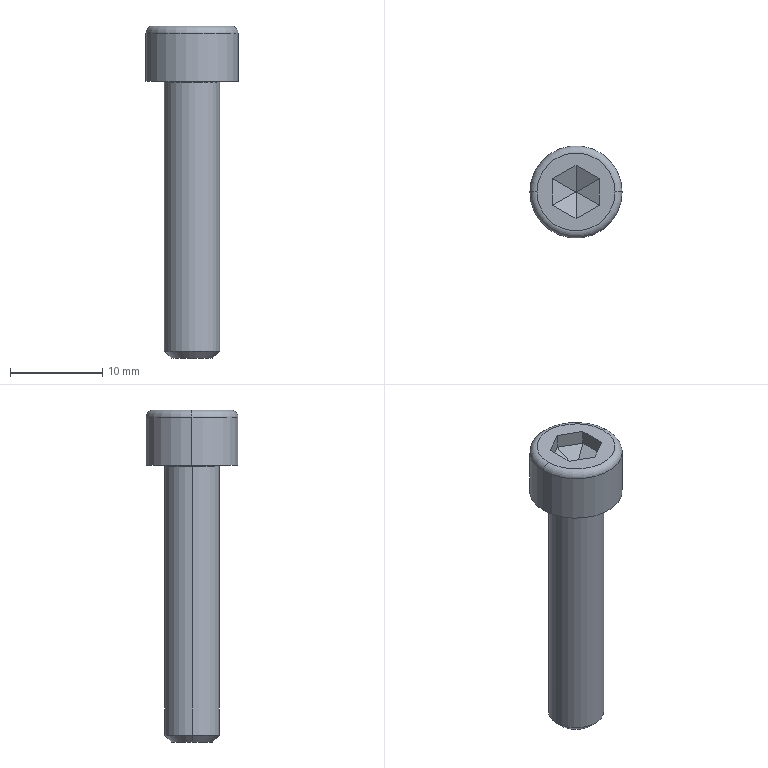Part | SolidWorks | features Chamfer 2, Fillet 2, ICE 2, Extrusion 1, RefAxis 1 | 1 solid | 26 faces | box 10 x 10 x 36 mm | volume 1267 mm3 | plane 16 | torus 4 | cylinder 4 | cone 2 | commonest cylinder face diameters 6 x2 10 x2
STEP:
#1=CARTESIAN_POINT('',(-3.1,0.,0.));
#2=VERTEX_POINT('',#1);
#3=CARTESIAN_POINT('',(3.1,0.,0.));
#4=VERTEX_POINT('',#3);
#5=CARTESIAN_POINT('',(0.,0.,0.));
#6=DIRECTION('',(0.,0.,1.));
#7=DIRECTION('',(1.,0.,0.));
#8=AXIS2_PLACEMENT_3D('',#5,#6,#7);
#9=CIRCLE('',#8,3.1);
#10=EDGE_CURVE('',#2,#4,#9,.T.);
#11=ORIENTED_EDGE('',*,*,#10,.F.);
#12=CARTESIAN_POINT('',(-3.,0.,-0.1));
#13=VERTEX_POINT('',#12);
#14=CARTESIAN_POINT('',(-3.1,0.,-0.1));
#15=DIRECTION('',(0.,1.,0.));
#16=DIRECTION('',(-1.,0.,0.));
#17=AXIS2_PLACEMENT_3D('',#14,#15,#16);
#18=CIRCLE('',#17,0.1);
#19=EDGE_CURVE('',#2,#13,#18,.T.);
#20=ORIENTED_EDGE('',*,*,#19,.T.);
#21=CARTESIAN_POINT('',(3.,0.,-0.1));
#22=VERTEX_POINT('',#21);
#23=CARTESIAN_POINT('',(0.,0.,-0.1));
#24=DIRECTION('',(0.,0.,-1.));
#25=DIRECTION('',(1.,0.,0.));
#26=AXIS2_PLACEMENT_3D('',#23,#24,#25);
#27=CIRCLE('',#26,3.);
#28=EDGE_CURVE('',#22,#13,#27,.T.);
#29=ORIENTED_EDGE('',*,*,#28,.F.);
#30=CARTESIAN_POINT('',(3.1,0.,-0.1));
#31=DIRECTION('',(0.,-1.,0.));
#32=DIRECTION('',(1.,0.,0.));
#33=AXIS2_PLACEMENT_3D('',#30,#31,#32);
#34=CIRCLE('',#33,0.1);
#35=EDGE_CURVE('',#4,#22,#34,.T.);
#36=ORIENTED_EDGE('',*,*,#35,.F.);
#37=EDGE_LOOP('',(#11,#20,#29,#36));
#38=FACE_OUTER_BOUND('',#37,.T.);
#39=CARTESIAN_POINT('',(0.,0.,-0.1));
#40=DIRECTION('',(0.,0.,1.));
#41=DIRECTION('',(1.,0.,0.));
#42=AXIS2_PLACEMENT_3D('',#39,#40,#41);
#43=TOROIDAL_SURFACE('',#42,3.1,0.1);
#44=ADVANCED_FACE('',(#38),#43,.F.);
#45=CARTESIAN_POINT('',(-5.,0.,5.231));
#46=VERTEX_POINT('',#45);
#47=CARTESIAN_POINT('',(5.,0.,5.231));
#48=VERTEX_POINT('',#47);
#49=CARTESIAN_POINT('',(0.,0.,5.231));
#50=DIRECTION('',(0.,0.,-1.));
#51=DIRECTION('',(1.,0.,0.));
#52=AXIS2_PLACEMENT_3D('',#49,#50,#51);
#53=CIRCLE('',#52,5.);
#54=EDGE_CURVE('',#46,#48,#53,.T.);
#55=ORIENTED_EDGE('',*,*,#54,.F.);
#56=CARTESIAN_POINT('',(-4.231,0.,6.));
#57=VERTEX_POINT('',#56);
#58=CARTESIAN_POINT('',(-4.231,0.,5.231));
#59=DIRECTION('',(0.,1.,0.));
#60=DIRECTION('',(-1.,0.,0.));
#61=AXIS2_PLACEMENT_3D('',#58,#59,#60);
#62=CIRCLE('',#61,0.7692);
#63=EDGE_CURVE('',#46,#57,#62,.T.);
#64=ORIENTED_EDGE('',*,*,#63,.T.);
#65=CARTESIAN_POINT('',(4.231,0.,6.));
#66=VERTEX_POINT('',#65);
#67=CARTESIAN_POINT('',(0.,0.,6.));
#68=DIRECTION('',(0.,0.,1.));
#69=DIRECTION('',(1.,0.,0.));
#70=AXIS2_PLACEMENT_3D('',#67,#68,#69);
#71=CIRCLE('',#70,4.231);
#72=EDGE_CURVE('',#66,#57,#71,.T.);
#73=ORIENTED_EDGE('',*,*,#72,.F.);
#74=CARTESIAN_POINT('',(4.231,0.,5.231));
#75=DIRECTION('',(0.,-1.,0.));
#76=DIRECTION('',(1.,0.,0.));
#77=AXIS2_PLACEMENT_3D('',#74,#75,#76);
#78=CIRCLE('',#77,0.7692);
#79=EDGE_CURVE('',#48,#66,#78,.T.);
#80=ORIENTED_EDGE('',*,*,#79,.F.);
#81=EDGE_LOOP('',(#55,#64,#73,#80));
#82=FACE_OUTER_BOUND('',#81,.T.);
#83=CARTESIAN_POINT('',(0.,0.,5.231));
#84=DIRECTION('',(0.,0.,1.));
#85=DIRECTION('',(1.,0.,0.));
#86=AXIS2_PLACEMENT_3D('',#83,#84,#85);
#87=TOROIDAL_SURFACE('',#86,4.231,0.7692);
#88=ADVANCED_FACE('',(#82),#87,.T.);
#89=CARTESIAN_POINT('',(-2.25,0.,-30.));
#90=VERTEX_POINT('',#89);
#91=CARTESIAN_POINT('',(2.25,0.,-30.));
#92=VERTEX_POINT('',#91);
#93=CARTESIAN_POINT('',(0.,0.,-30.));
#94=DIRECTION('',(0.,0.,-1.));
#95=DIRECTION('',(-1.,0.,0.));
#96=AXIS2_PLACEMENT_3D('',#93,#94,#95);
#97=CIRCLE('',#96,2.25);
#98=EDGE_CURVE('',#90,#92,#97,.T.);
#99=ORIENTED_EDGE('',*,*,#98,.F.);
#100=CARTESIAN_POINT('',(-3.,0.,-29.25));
#101=VERTEX_POINT('',#100);
#102=CARTESIAN_POINT('',(-2.25,0.,-30.));
#103=DIRECTION('',(-0.7071,0.,0.7071));
#104=VECTOR('',#103,1000.);
#105=LINE('',#102,#104);
#106=EDGE_CURVE('',#90,#101,#105,.T.);
#107=ORIENTED_EDGE('',*,*,#106,.T.);
#108=CARTESIAN_POINT('',(3.,0.,-29.25));
#109=VERTEX_POINT('',#108);
#110=CARTESIAN_POINT('',(0.,0.,-29.25));
#111=DIRECTION('',(0.,0.,1.));
#112=DIRECTION('',(-1.,0.,0.));
#113=AXIS2_PLACEMENT_3D('',#110,#111,#112);
#114=CIRCLE('',#113,3.);
#115=EDGE_CURVE('',#109,#101,#114,.T.);
#116=ORIENTED_EDGE('',*,*,#115,.F.);
#117=CARTESIAN_POINT('',(2.25,0.,-30.));
#118=DIRECTION('',(0.7071,0.,0.7071));
#119=VECTOR('',#118,1000.);
#120=LINE('',#117,#119);
#121=EDGE_CURVE('',#92,#109,#120,.T.);
#122=ORIENTED_EDGE('',*,*,#121,.F.);
#123=EDGE_LOOP('',(#99,#107,#116,#122));
#124=FACE_OUTER_BOUND('',#123,.T.);
#125=CARTESIAN_POINT('',(0.,0.,-30.));
#126=DIRECTION('',(0.,0.,1.));
#127=DIRECTION('',(1.,0.,0.));
#128=AXIS2_PLACEMENT_3D('',#125,#126,#127);
#129=CONICAL_SURFACE('',#128,2.25,0.7854);
#130=ADVANCED_FACE('',(#124),#129,.T.);
#131=ORIENTED_EDGE('',*,*,#115,.T.);
#132=CARTESIAN_POINT('',(-3.,0.,-30.));
#133=DIRECTION('',(0.,0.,1.));
#134=VECTOR('',#133,1000.);
#135=LINE('',#132,#134);
#136=EDGE_CURVE('',#101,#13,#135,.T.);
#137=ORIENTED_EDGE('',*,*,#136,.T.);
#138=CARTESIAN_POINT('',(0.,0.,-0.1));
#139=DIRECTION('',(0.,0.,-1.));
#140=DIRECTION('',(1.,0.,0.));
#141=AXIS2_PLACEMENT_3D('',#138,#139,#140);
#142=CIRCLE('',#141,3.);
#143=EDGE_CURVE('',#13,#22,#142,.T.);
#144=ORIENTED_EDGE('',*,*,#143,.T.);
#145=CARTESIAN_POINT('',(3.,0.,-30.));
#146=DIRECTION('',(0.,0.,1.));
#147=VECTOR('',#146,1000.);
#148=LINE('',#145,#147);
#149=EDGE_CURVE('',#109,#22,#148,.T.);
#150=ORIENTED_EDGE('',*,*,#149,.F.);
#151=EDGE_LOOP('',(#131,#137,#144,#150));
#152=FACE_OUTER_BOUND('',#151,.T.);
#153=CARTESIAN_POINT('',(0.,0.,-30.));
#154=DIRECTION('',(0.,0.,1.));
#155=DIRECTION('',(1.,0.,0.));
#156=AXIS2_PLACEMENT_3D('',#153,#154,#155);
#157=CYLINDRICAL_SURFACE('',#156,3.);
#158=ADVANCED_FACE('',(#152),#157,.T.);
#159=ORIENTED_EDGE('',*,*,#54,.T.);
#160=CARTESIAN_POINT('',(5.,0.,0.));
#161=VERTEX_POINT('',#160);
#162=CARTESIAN_POINT('',(5.,0.,6.));
#163=DIRECTION('',(0.,0.,-1.));
#164=VECTOR('',#163,1000.);
#165=LINE('',#162,#164);
#166=EDGE_CURVE('',#48,#161,#165,.T.);
#167=ORIENTED_EDGE('',*,*,#166,.T.);
#168=CARTESIAN_POINT('',(-5.,0.,0.));
#169=VERTEX_POINT('',#168);
#170=CARTESIAN_POINT('',(0.,0.,0.));
#171=DIRECTION('',(0.,0.,1.));
#172=DIRECTION('',(1.,0.,0.));
#173=AXIS2_PLACEMENT_3D('',#170,#171,#172);
#174=CIRCLE('',#173,5.);
#175=EDGE_CURVE('',#161,#169,#174,.T.);
#176=ORIENTED_EDGE('',*,*,#175,.T.);
#177=CARTESIAN_POINT('',(-5.,0.,6.));
#178=DIRECTION('',(0.,0.,-1.));
#179=VECTOR('',#178,1000.);
#180=LINE('',#177,#179);
#181=EDGE_CURVE('',#46,#169,#180,.T.);
#182=ORIENTED_EDGE('',*,*,#181,.F.);
#183=EDGE_LOOP('',(#159,#167,#176,#182));
#184=FACE_OUTER_BOUND('',#183,.T.);
#185=CARTESIAN_POINT('',(0.,0.,6.));
#186=DIRECTION('',(0.,0.,-1.));
#187=DIRECTION('',(-1.,0.,0.));
#188=AXIS2_PLACEMENT_3D('',#185,#186,#187);
#189=CYLINDRICAL_SURFACE('',#188,5.);
#190=ADVANCED_FACE('',(#184),#189,.T.);
#191=CARTESIAN_POINT('',(0.,0.,0.));
#192=DIRECTION('',(0.,0.,1.));
#193=DIRECTION('',(1.,0.,0.));
#194=AXIS2_PLACEMENT_3D('',#191,#192,#193);
#195=CIRCLE('',#194,3.1);
#196=EDGE_CURVE('',#4,#2,#195,.T.);
#197=ORIENTED_EDGE('',*,*,#196,.T.);
#198=ORIENTED_EDGE('',*,*,#10,.T.);
#199=EDGE_LOOP('',(#197,#198));
#200=FACE_BOUND('',#199,.T.);
#201=CARTESIAN_POINT('',(0.,0.,0.));
#202=DIRECTION('',(0.,0.,1.));
#203=DIRECTION('',(1.,0.,0.));
#204=AXIS2_PLACEMENT_3D('',#201,#202,#203);
#205=CIRCLE('',#204,5.);
#206=EDGE_CURVE('',#169,#161,#205,.T.);
#207=ORIENTED_EDGE('',*,*,#206,.F.);
#208=ORIENTED_EDGE('',*,*,#175,.F.);
#209=EDGE_LOOP('',(#207,#208));
#210=FACE_OUTER_BOUND('',#209,.T.);
#211=CARTESIAN_POINT('',(0.,0.,0.));
#212=DIRECTION('',(0.,0.,1.));
#213=DIRECTION('',(1.,0.,0.));
#214=AXIS2_PLACEMENT_3D('',#211,#212,#213);
#215=PLANE('',#214);
#216=ADVANCED_FACE('',(#200,#210),#215,.F.);
#217=ORIENTED_EDGE('',*,*,#166,.F.);
#218=CARTESIAN_POINT('',(0.,0.,5.231));
#219=DIRECTION('',(0.,0.,-1.));
#220=DIRECTION('',(1.,0.,0.));
#221=AXIS2_PLACEMENT_3D('',#218,#219,#220);
#222=CIRCLE('',#221,5.);
#223=EDGE_CURVE('',#48,#46,#222,.T.);
#224=ORIENTED_EDGE('',*,*,#223,.T.);
#225=ORIENTED_EDGE('',*,*,#181,.T.);
#226=ORIENTED_EDGE('',*,*,#206,.T.);
#227=EDGE_LOOP('',(#217,#224,#225,#226));
#228=FACE_OUTER_BOUND('',#227,.T.);
#229=CARTESIAN_POINT('',(0.,0.,6.));
#230=DIRECTION('',(0.,0.,-1.));
#231=DIRECTION('',(-1.,0.,0.));
#232=AXIS2_PLACEMENT_3D('',#229,#230,#231);
#233=CYLINDRICAL_SURFACE('',#232,5.);
#234=ADVANCED_FACE('',(#228),#233,.T.);
#235=ORIENTED_EDGE('',*,*,#72,.T.);
#236=CARTESIAN_POINT('',(0.,0.,6.));
#237=DIRECTION('',(0.,0.,1.));
#238=DIRECTION('',(1.,0.,0.));
#239=AXIS2_PLACEMENT_3D('',#236,#237,#238);
#240=CIRCLE('',#239,4.231);
#241=EDGE_CURVE('',#57,#66,#240,.T.);
#242=ORIENTED_EDGE('',*,*,#241,.T.);
#243=EDGE_LOOP('',(#235,#242));
#244=FACE_OUTER_BOUND('',#243,.T.);
#245=CARTESIAN_POINT('',(2.5,-1.443,6.));
#246=VERTEX_POINT('',#245);
#247=CARTESIAN_POINT('',(2.5,1.443,6.));
#248=VERTEX_POINT('',#247);
#249=CARTESIAN_POINT('',(2.5,-1.443,6.));
#250=DIRECTION('',(0.,1.,0.));
#251=VECTOR('',#250,1000.);
#252=LINE('',#249,#251);
#253=EDGE_CURVE('',#246,#248,#252,.T.);
#254=ORIENTED_EDGE('',*,*,#253,.F.);
#255=CARTESIAN_POINT('',(0.,-2.887,6.));
#256=VERTEX_POINT('',#255);
#257=CARTESIAN_POINT('',(0.,-2.887,6.));
#258=DIRECTION('',(0.866,0.5,0.));
#259=VECTOR('',#258,1000.);
#260=LINE('',#257,#259);
#261=EDGE_CURVE('',#256,#246,#260,.T.);
#262=ORIENTED_EDGE('',*,*,#261,.F.);
#263=CARTESIAN_POINT('',(-2.5,-1.443,6.));
#264=VERTEX_POINT('',#263);
#265=CARTESIAN_POINT('',(-2.5,-1.443,6.));
#266=DIRECTION('',(0.866,-0.5,0.));
#267=VECTOR('',#266,1000.);
#268=LINE('',#265,#267);
#269=EDGE_CURVE('',#264,#256,#268,.T.);
#270=ORIENTED_EDGE('',*,*,#269,.F.);
#271=CARTESIAN_POINT('',(-2.5,1.443,6.));
#272=VERTEX_POINT('',#271);
#273=CARTESIAN_POINT('',(-2.5,1.443,6.));
#274=DIRECTION('',(0.,-1.,0.));
#275=VECTOR('',#274,1000.);
#276=LINE('',#273,#275);
#277=EDGE_CURVE('',#272,#264,#276,.T.);
#278=ORIENTED_EDGE('',*,*,#277,.F.);
#279=CARTESIAN_POINT('',(0.,2.887,6.));
#280=VERTEX_POINT('',#279);
#281=CARTESIAN_POINT('',(0.,2.887,6.));
#282=DIRECTION('',(-0.866,-0.5,0.));
#283=VECTOR('',#282,1000.);
#284=LINE('',#281,#283);
#285=EDGE_CURVE('',#280,#272,#284,.T.);
#286=ORIENTED_EDGE('',*,*,#285,.F.);
#287=CARTESIAN_POINT('',(2.5,1.443,6.));
#288=DIRECTION('',(-0.866,0.5,0.));
#289=VECTOR('',#288,1000.);
#290=LINE('',#287,#289);
#291=EDGE_CURVE('',#248,#280,#290,.T.);
#292=ORIENTED_EDGE('',*,*,#291,.F.);
#293=EDGE_LOOP('',(#254,#262,#270,#278,#286,#292));
#294=FACE_BOUND('',#293,.T.);
#295=CARTESIAN_POINT('',(0.,0.,6.));
#296=DIRECTION('',(0.,0.,1.));
#297=DIRECTION('',(1.,0.,0.));
#298=AXIS2_PLACEMENT_3D('',#295,#296,#297);
#299=PLANE('',#298);
#300=ADVANCED_FACE('',(#244,#294),#299,.T.);
#301=CARTESIAN_POINT('',(2.5,1.443,4.441));
#302=VERTEX_POINT('',#301);
#303=CARTESIAN_POINT('',(2.5,1.443,3.));
#304=DIRECTION('',(0.,0.,1.));
#305=VECTOR('',#304,1000.);
#306=LINE('',#303,#305);
#307=EDGE_CURVE('',#302,#248,#306,.T.);
#308=ORIENTED_EDGE('',*,*,#307,.F.);
#309=CARTESIAN_POINT('',(2.5,-1.443,4.441));
#310=VERTEX_POINT('',#309);
#311=CARTESIAN_POINT('',(2.5,-1.443,4.441));
#312=DIRECTION('',(0.,-1.,0.));
#313=VECTOR('',#312,1000.);
#314=LINE('',#311,#313);
#315=EDGE_CURVE('',#302,#310,#314,.T.);
#316=ORIENTED_EDGE('',*,*,#315,.T.);
#317=CARTESIAN_POINT('',(2.5,-1.443,3.));
#318=DIRECTION('',(0.,0.,1.));
#319=VECTOR('',#318,1000.);
#320=LINE('',#317,#319);
#321=EDGE_CURVE('',#310,#246,#320,.T.);
#322=ORIENTED_EDGE('',*,*,#321,.T.);
#323=ORIENTED_EDGE('',*,*,#253,.T.);
#324=EDGE_LOOP('',(#308,#316,#322,#323));
#325=FACE_OUTER_BOUND('',#324,.T.);
#326=CARTESIAN_POINT('',(2.5,-1.443,3.));
#327=DIRECTION('',(1.,0.,0.));
#328=DIRECTION('',(0.,0.,-1.));
#329=AXIS2_PLACEMENT_3D('',#326,#327,#328);
#330=PLANE('',#329);
#331=ADVANCED_FACE('',(#325),#330,.F.);
#332=ORIENTED_EDGE('',*,*,#321,.F.);
#333=CARTESIAN_POINT('',(0.,-2.887,4.441));
#334=VERTEX_POINT('',#333);
#335=CARTESIAN_POINT('',(0.,-2.887,4.441));
#336=DIRECTION('',(-0.866,-0.5,0.));
#337=VECTOR('',#336,1000.);
#338=LINE('',#335,#337);
#339=EDGE_CURVE('',#310,#334,#338,.T.);
#340=ORIENTED_EDGE('',*,*,#339,.T.);
#341=CARTESIAN_POINT('',(0.,-2.887,3.));
#342=DIRECTION('',(0.,0.,1.));
#343=VECTOR('',#342,1000.);
#344=LINE('',#341,#343);
#345=EDGE_CURVE('',#334,#256,#344,.T.);
#346=ORIENTED_EDGE('',*,*,#345,.T.);
#347=ORIENTED_EDGE('',*,*,#261,.T.);
#348=EDGE_LOOP('',(#332,#340,#346,#347));
#349=FACE_OUTER_BOUND('',#348,.T.);
#350=CARTESIAN_POINT('',(0.,-2.887,3.));
#351=DIRECTION('',(0.5,-0.866,0.));
#352=DIRECTION('',(0.866,0.5,0.));
#353=AXIS2_PLACEMENT_3D('',#350,#351,#352);
#354=PLANE('',#353);
#355=ADVANCED_FACE('',(#349),#354,.F.);
#356=ORIENTED_EDGE('',*,*,#345,.F.);
#357=CARTESIAN_POINT('',(-2.5,-1.443,4.441));
#358=VERTEX_POINT('',#357);
#359=CARTESIAN_POINT('',(-2.5,-1.443,4.441));
#360=DIRECTION('',(-0.866,0.5,0.));
#361=VECTOR('',#360,1000.);
#362=LINE('',#359,#361);
#363=EDGE_CURVE('',#334,#358,#362,.T.);
#364=ORIENTED_EDGE('',*,*,#363,.T.);
#365=CARTESIAN_POINT('',(-2.5,-1.443,3.));
#366=DIRECTION('',(0.,0.,1.));
#367=VECTOR('',#366,1000.);
#368=LINE('',#365,#367);
#369=EDGE_CURVE('',#358,#264,#368,.T.);
#370=ORIENTED_EDGE('',*,*,#369,.T.);
#371=ORIENTED_EDGE('',*,*,#269,.T.);
#372=EDGE_LOOP('',(#356,#364,#370,#371));
#373=FACE_OUTER_BOUND('',#372,.T.);
#374=CARTESIAN_POINT('',(-2.5,-1.443,3.));
#375=DIRECTION('',(-0.5,-0.866,0.));
#376=DIRECTION('',(0.866,-0.5,0.));
#377=AXIS2_PLACEMENT_3D('',#374,#375,#376);
#378=PLANE('',#377);
#379=ADVANCED_FACE('',(#373),#378,.F.);
#380=ORIENTED_EDGE('',*,*,#369,.F.);
#381=CARTESIAN_POINT('',(-2.5,1.443,4.441));
#382=VERTEX_POINT('',#381);
#383=CARTESIAN_POINT('',(-2.5,1.443,4.441));
#384=DIRECTION('',(0.,1.,0.));
#385=VECTOR('',#384,1000.);
#386=LINE('',#383,#385);
#387=EDGE_CURVE('',#358,#382,#386,.T.);
#388=ORIENTED_EDGE('',*,*,#387,.T.);
#389=CARTESIAN_POINT('',(-2.5,1.443,3.));
#390=DIRECTION('',(0.,0.,1.));
#391=VECTOR('',#390,1000.);
#392=LINE('',#389,#391);
#393=EDGE_CURVE('',#382,#272,#392,.T.);
#394=ORIENTED_EDGE('',*,*,#393,.T.);
#395=ORIENTED_EDGE('',*,*,#277,.T.);
#396=EDGE_LOOP('',(#380,#388,#394,#395));
#397=FACE_OUTER_BOUND('',#396,.T.);
#398=CARTESIAN_POINT('',(-2.5,1.443,3.));
#399=DIRECTION('',(-1.,0.,0.));
#400=DIRECTION('',(0.,0.,1.));
#401=AXIS2_PLACEMENT_3D('',#398,#399,#400);
#402=PLANE('',#401);
#403=ADVANCED_FACE('',(#397),#402,.F.);
#404=ORIENTED_EDGE('',*,*,#393,.F.);
#405=CARTESIAN_POINT('',(0.,2.887,4.441));
#406=VERTEX_POINT('',#405);
#407=CARTESIAN_POINT('',(0.,2.887,4.441));
#408=DIRECTION('',(0.866,0.5,0.));
#409=VECTOR('',#408,1000.);
#410=LINE('',#407,#409);
#411=EDGE_CURVE('',#382,#406,#410,.T.);
#412=ORIENTED_EDGE('',*,*,#411,.T.);
#413=CARTESIAN_POINT('',(0.,2.887,3.));
#414=DIRECTION('',(0.,0.,1.));
#415=VECTOR('',#414,1000.);
#416=LINE('',#413,#415);
#417=EDGE_CURVE('',#406,#280,#416,.T.);
#418=ORIENTED_EDGE('',*,*,#417,.T.);
#419=ORIENTED_EDGE('',*,*,#285,.T.);
#420=EDGE_LOOP('',(#404,#412,#418,#419));
#421=FACE_OUTER_BOUND('',#420,.T.);
#422=CARTESIAN_POINT('',(0.,2.887,3.));
#423=DIRECTION('',(-0.5,0.866,0.));
#424=DIRECTION('',(-0.866,-0.5,0.));
#425=AXIS2_PLACEMENT_3D('',#422,#423,#424);
#426=PLANE('',#425);
#427=ADVANCED_FACE('',(#421),#426,.F.);
#428=ORIENTED_EDGE('',*,*,#417,.F.);
#429=CARTESIAN_POINT('',(2.5,1.443,4.441));
#430=DIRECTION('',(0.866,-0.5,0.));
#431=VECTOR('',#430,1000.);
#432=LINE('',#429,#431);
#433=EDGE_CURVE('',#406,#302,#432,.T.);
#434=ORIENTED_EDGE('',*,*,#433,.T.);
#435=ORIENTED_EDGE('',*,*,#307,.T.);
#436=ORIENTED_EDGE('',*,*,#291,.T.);
#437=EDGE_LOOP('',(#428,#434,#435,#436));
#438=FACE_OUTER_BOUND('',#437,.T.);
#439=CARTESIAN_POINT('',(2.5,1.443,3.));
#440=DIRECTION('',(0.5,0.866,0.));
#441=DIRECTION('',(-0.866,0.5,0.));
#442=AXIS2_PLACEMENT_3D('',#439,#440,#441);
#443=PLANE('',#442);
#444=ADVANCED_FACE('',(#438),#443,.F.);
#445=CARTESIAN_POINT('',(0.,0.004907,3.));
#446=VERTEX_POINT('',#445);
#447=CARTESIAN_POINT('',(-0.00425,0.002453,3.));
#448=VERTEX_POINT('',#447);
#449=CARTESIAN_POINT('',(-0.002125,0.00368,3.));
#450=DIRECTION('',(-0.866,-0.5,0.));
#451=VECTOR('',#450,1000.);
#452=LINE('',#449,#451);
#453=EDGE_CURVE('',#446,#448,#452,.T.);
#454=ORIENTED_EDGE('',*,*,#453,.T.);
#455=CARTESIAN_POINT('',(-0.00425,-0.002453,3.));
#456=VERTEX_POINT('',#455);
#457=CARTESIAN_POINT('',(-0.00425,0.,3.));
#458=DIRECTION('',(0.,-1.,0.));
#459=VECTOR('',#458,1000.);
#460=LINE('',#457,#459);
#461=EDGE_CURVE('',#448,#456,#460,.T.);
#462=ORIENTED_EDGE('',*,*,#461,.T.);
#463=CARTESIAN_POINT('',(0.,-0.004907,3.));
#464=VERTEX_POINT('',#463);
#465=CARTESIAN_POINT('',(-0.002125,-0.00368,3.));
#466=DIRECTION('',(0.866,-0.5,0.));
#467=VECTOR('',#466,1000.);
#468=LINE('',#465,#467);
#469=EDGE_CURVE('',#456,#464,#468,.T.);
#470=ORIENTED_EDGE('',*,*,#469,.T.);
#471=CARTESIAN_POINT('',(0.00425,-0.002453,3.));
#472=VERTEX_POINT('',#471);
#473=CARTESIAN_POINT('',(0.002125,-0.00368,3.));
#474=DIRECTION('',(0.866,0.5,0.));
#475=VECTOR('',#474,1000.);
#476=LINE('',#473,#475);
#477=EDGE_CURVE('',#464,#472,#476,.T.);
#478=ORIENTED_EDGE('',*,*,#477,.T.);
#479=CARTESIAN_POINT('',(0.00425,0.002453,3.));
#480=VERTEX_POINT('',#479);
#481=CARTESIAN_POINT('',(0.00425,0.,3.));
#482=DIRECTION('',(0.,1.,0.));
#483=VECTOR('',#482,1000.);
#484=LINE('',#481,#483);
#485=EDGE_CURVE('',#472,#480,#484,.T.);
#486=ORIENTED_EDGE('',*,*,#485,.T.);
#487=CARTESIAN_POINT('',(0.002125,0.00368,3.));
#488=DIRECTION('',(-0.866,0.5,0.));
#489=VECTOR('',#488,1000.);
#490=LINE('',#487,#489);
#491=EDGE_CURVE('',#480,#446,#490,.T.);
#492=ORIENTED_EDGE('',*,*,#491,.T.);
#493=EDGE_LOOP('',(#454,#462,#470,#478,#486,#492));
#494=FACE_OUTER_BOUND('',#493,.T.);
#495=CARTESIAN_POINT('',(0.,0.,3.));
#496=DIRECTION('',(0.,0.,1.));
#497=DIRECTION('',(1.,0.,0.));
#498=AXIS2_PLACEMENT_3D('',#495,#496,#497);
#499=PLANE('',#498);
#500=ADVANCED_FACE('',(#494),#499,.T.);
#501=ORIENTED_EDGE('',*,*,#136,.F.);
#502=CARTESIAN_POINT('',(0.,0.,-29.25));
#503=DIRECTION('',(0.,0.,1.));
#504=DIRECTION('',(-1.,0.,0.));
#505=AXIS2_PLACEMENT_3D('',#502,#503,#504);
#506=CIRCLE('',#505,3.);
#507=EDGE_CURVE('',#101,#109,#506,.T.);
#508=ORIENTED_EDGE('',*,*,#507,.T.);
#509=ORIENTED_EDGE('',*,*,#149,.T.);
#510=ORIENTED_EDGE('',*,*,#28,.T.);
#511=EDGE_LOOP('',(#501,#508,#509,#510));
#512=FACE_OUTER_BOUND('',#511,.T.);
#513=CARTESIAN_POINT('',(0.,0.,-30.));
#514=DIRECTION('',(0.,0.,1.));
#515=DIRECTION('',(1.,0.,0.));
#516=AXIS2_PLACEMENT_3D('',#513,#514,#515);
#517=CYLINDRICAL_SURFACE('',#516,3.);
#518=ADVANCED_FACE('',(#512),#517,.T.);
#519=CARTESIAN_POINT('',(0.,0.,-30.));
#520=DIRECTION('',(0.,0.,-1.));
#521=DIRECTION('',(-1.,0.,0.));
#522=AXIS2_PLACEMENT_3D('',#519,#520,#521);
#523=CIRCLE('',#522,2.25);
#524=EDGE_CURVE('',#92,#90,#523,.T.);
#525=ORIENTED_EDGE('',*,*,#524,.T.);
#526=ORIENTED_EDGE('',*,*,#98,.T.);
#527=EDGE_LOOP('',(#525,#526));
#528=FACE_OUTER_BOUND('',#527,.T.);
#529=CARTESIAN_POINT('',(0.,0.,-30.));
#530=DIRECTION('',(0.,0.,-1.));
#531=DIRECTION('',(-1.,0.,0.));
#532=AXIS2_PLACEMENT_3D('',#529,#530,#531);
#533=PLANE('',#532);
#534=ADVANCED_FACE('',(#528),#533,.T.);
#535=ORIENTED_EDGE('',*,*,#106,.F.);
#536=ORIENTED_EDGE('',*,*,#524,.F.);
#537=ORIENTED_EDGE('',*,*,#121,.T.);
#538=ORIENTED_EDGE('',*,*,#507,.F.);
#539=EDGE_LOOP('',(#535,#536,#537,#538));
#540=FACE_OUTER_BOUND('',#539,.T.);
#541=CARTESIAN_POINT('',(0.,0.,-30.));
#542=DIRECTION('',(0.,0.,1.));
#543=DIRECTION('',(1.,0.,0.));
#544=AXIS2_PLACEMENT_3D('',#541,#542,#543);
#545=CONICAL_SURFACE('',#544,2.25,0.7854);
#546=ADVANCED_FACE('',(#540),#545,.T.);
#547=ORIENTED_EDGE('',*,*,#63,.F.);
#548=ORIENTED_EDGE('',*,*,#223,.F.);
#549=ORIENTED_EDGE('',*,*,#79,.T.);
#550=ORIENTED_EDGE('',*,*,#241,.F.);
#551=EDGE_LOOP('',(#547,#548,#549,#550));
#552=FACE_OUTER_BOUND('',#551,.T.);
#553=CARTESIAN_POINT('',(0.,0.,5.231));
#554=DIRECTION('',(0.,0.,1.));
#555=DIRECTION('',(1.,0.,0.));
#556=AXIS2_PLACEMENT_3D('',#553,#554,#555);
#557=TOROIDAL_SURFACE('',#556,4.231,0.7692);
#558=ADVANCED_FACE('',(#552),#557,.T.);
#559=CARTESIAN_POINT('',(0.0034,-0.001963,3.));
#560=DIRECTION('',(-0.7746,0.4472,-0.4472));
#561=VECTOR('',#560,1000.);
#562=LINE('',#559,#561);
#563=EDGE_CURVE('',#310,#472,#562,.T.);
#564=ORIENTED_EDGE('',*,*,#563,.F.);
#565=ORIENTED_EDGE('',*,*,#315,.F.);
#566=CARTESIAN_POINT('',(0.0034,0.001963,3.));
#567=DIRECTION('',(0.7746,0.4472,0.4472));
#568=VECTOR('',#567,1000.);
#569=LINE('',#566,#568);
#570=EDGE_CURVE('',#480,#302,#569,.T.);
#571=ORIENTED_EDGE('',*,*,#570,.F.);
#572=ORIENTED_EDGE('',*,*,#485,.F.);
#573=EDGE_LOOP('',(#564,#565,#571,#572));
#574=FACE_OUTER_BOUND('',#573,.T.);
#575=CARTESIAN_POINT('',(0.00425,0.,3.));
#576=DIRECTION('',(0.5,0.,-0.866));
#577=DIRECTION('',(0.,1.,0.));
#578=AXIS2_PLACEMENT_3D('',#575,#576,#577);
#579=PLANE('',#578);
#580=ADVANCED_FACE('',(#574),#579,.F.);
#581=ORIENTED_EDGE('',*,*,#570,.T.);
#582=ORIENTED_EDGE('',*,*,#433,.F.);
#583=CARTESIAN_POINT('',(0.,0.003926,3.));
#584=DIRECTION('',(0.,0.8944,0.4472));
#585=VECTOR('',#584,1000.);
#586=LINE('',#583,#585);
#587=EDGE_CURVE('',#446,#406,#586,.T.);
#588=ORIENTED_EDGE('',*,*,#587,.F.);
#589=ORIENTED_EDGE('',*,*,#491,.F.);
#590=EDGE_LOOP('',(#581,#582,#588,#589));
#591=FACE_OUTER_BOUND('',#590,.T.);
#592=CARTESIAN_POINT('',(0.002125,0.00368,3.));
#593=DIRECTION('',(0.25,0.433,-0.866));
#594=DIRECTION('',(-0.866,0.5,0.));
#595=AXIS2_PLACEMENT_3D('',#592,#593,#594);
#596=PLANE('',#595);
#597=ADVANCED_FACE('',(#591),#596,.F.);
#598=ORIENTED_EDGE('',*,*,#563,.T.);
#599=ORIENTED_EDGE('',*,*,#477,.F.);
#600=CARTESIAN_POINT('',(0.,-0.003926,3.));
#601=DIRECTION('',(0.,0.8944,-0.4472));
#602=VECTOR('',#601,1000.);
#603=LINE('',#600,#602);
#604=EDGE_CURVE('',#334,#464,#603,.T.);
#605=ORIENTED_EDGE('',*,*,#604,.F.);
#606=ORIENTED_EDGE('',*,*,#339,.F.);
#607=EDGE_LOOP('',(#598,#599,#605,#606));
#608=FACE_OUTER_BOUND('',#607,.T.);
#609=CARTESIAN_POINT('',(0.002125,-0.00368,3.));
#610=DIRECTION('',(0.25,-0.433,-0.866));
#611=DIRECTION('',(0.866,0.5,0.));
#612=AXIS2_PLACEMENT_3D('',#609,#610,#611);
#613=PLANE('',#612);
#614=ADVANCED_FACE('',(#608),#613,.F.);
#615=ORIENTED_EDGE('',*,*,#587,.T.);
#616=ORIENTED_EDGE('',*,*,#411,.F.);
#617=CARTESIAN_POINT('',(-0.0034,0.001963,3.));
#618=DIRECTION('',(-0.7746,0.4472,0.4472));
#619=VECTOR('',#618,1000.);
#620=LINE('',#617,#619);
#621=EDGE_CURVE('',#448,#382,#620,.T.);
#622=ORIENTED_EDGE('',*,*,#621,.F.);
#623=ORIENTED_EDGE('',*,*,#453,.F.);
#624=EDGE_LOOP('',(#615,#616,#622,#623));
#625=FACE_OUTER_BOUND('',#624,.T.);
#626=CARTESIAN_POINT('',(-0.002125,0.00368,3.));
#627=DIRECTION('',(-0.25,0.433,-0.866));
#628=DIRECTION('',(-0.866,-0.5,0.));
#629=AXIS2_PLACEMENT_3D('',#626,#627,#628);
#630=PLANE('',#629);
#631=ADVANCED_FACE('',(#625),#630,.F.);
#632=ORIENTED_EDGE('',*,*,#604,.T.);
#633=ORIENTED_EDGE('',*,*,#469,.F.);
#634=CARTESIAN_POINT('',(-0.0034,-0.001963,3.));
#635=DIRECTION('',(0.7746,0.4472,-0.4472));
#636=VECTOR('',#635,1000.);
#637=LINE('',#634,#636);
#638=EDGE_CURVE('',#358,#456,#637,.T.);
#639=ORIENTED_EDGE('',*,*,#638,.F.);
#640=ORIENTED_EDGE('',*,*,#363,.F.);
#641=EDGE_LOOP('',(#632,#633,#639,#640));
#642=FACE_OUTER_BOUND('',#641,.T.);
#643=CARTESIAN_POINT('',(-0.002125,-0.00368,3.));
#644=DIRECTION('',(-0.25,-0.433,-0.866));
#645=DIRECTION('',(0.866,-0.5,0.));
#646=AXIS2_PLACEMENT_3D('',#643,#644,#645);
#647=PLANE('',#646);
#648=ADVANCED_FACE('',(#642),#647,.F.);
#649=ORIENTED_EDGE('',*,*,#621,.T.);
#650=ORIENTED_EDGE('',*,*,#387,.F.);
#651=ORIENTED_EDGE('',*,*,#638,.T.);
#652=ORIENTED_EDGE('',*,*,#461,.F.);
#653=EDGE_LOOP('',(#649,#650,#651,#652));
#654=FACE_OUTER_BOUND('',#653,.T.);
#655=CARTESIAN_POINT('',(-0.00425,0.,3.));
#656=DIRECTION('',(-0.5,0.,-0.866));
#657=DIRECTION('',(0.,-1.,0.));
#658=AXIS2_PLACEMENT_3D('',#655,#656,#657);
#659=PLANE('',#658);
#660=ADVANCED_FACE('',(#654),#659,.F.);
#661=ORIENTED_EDGE('',*,*,#19,.F.);
#662=ORIENTED_EDGE('',*,*,#196,.F.);
#663=ORIENTED_EDGE('',*,*,#35,.T.);
#664=ORIENTED_EDGE('',*,*,#143,.F.);
#665=EDGE_LOOP('',(#661,#662,#663,#664));
#666=FACE_OUTER_BOUND('',#665,.T.);
#667=CARTESIAN_POINT('',(0.,0.,-0.1));
#668=DIRECTION('',(0.,0.,1.));
#669=DIRECTION('',(1.,0.,0.));
#670=AXIS2_PLACEMENT_3D('',#667,#668,#669);
#671=TOROIDAL_SURFACE('',#670,3.1,0.1);
#672=ADVANCED_FACE('',(#666),#671,.F.);
#673=CLOSED_SHELL('',(#44,#88,#130,#158,#190,#216,#234,#300,#331,#355,#379,#403,#427,#444,#500,#518,#534,#546,#558,#580,#597,#614,#631,#648,#660,#672));
#674=MANIFOLD_SOLID_BREP('',#673);
#675=CARTESIAN_POINT('',(0.,0.,0.));
#676=DIRECTION('',(0.,0.,1.));
#677=DIRECTION('',(1.,0.,0.));
#678=AXIS2_PLACEMENT_3D('',#675,#676,#677);
#679=(LENGTH_UNIT()NAMED_UNIT(*)SI_UNIT(.MILLI.,.METRE.));
#680=UNCERTAINTY_MEASURE_WITH_UNIT(LENGTH_MEASURE(0.00001),#679,'','');
#681=(NAMED_UNIT(*)PLANE_ANGLE_UNIT()SI_UNIT($,.RADIAN.));
#682=(NAMED_UNIT(*)SI_UNIT($,.STERADIAN.)SOLID_ANGLE_UNIT());
#683=(GEOMETRIC_REPRESENTATION_CONTEXT(3)GLOBAL_UNCERTAINTY_ASSIGNED_CONTEXT((#680))GLOBAL_UNIT_ASSIGNED_CONTEXT((#679,#681,#682))REPRESENTATION_CONTEXT('',''));
#684=ADVANCED_BREP_SHAPE_REPRESENTATION('',(#674,#678),#683);